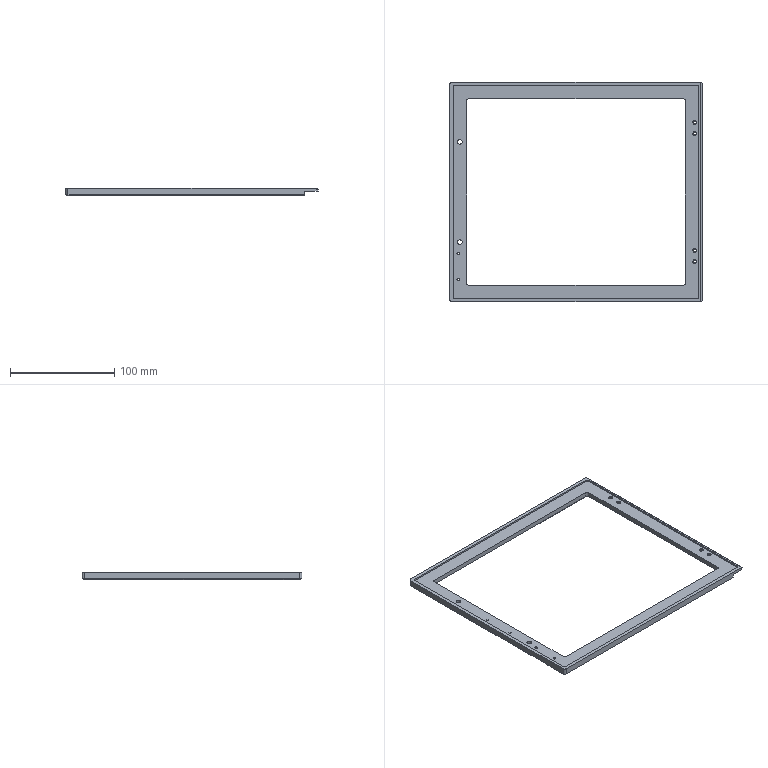NC program | NX | posted with a generic post | part box 241.5 x 210.5 x 7 mm
Lines 1 to 415 of 3179:
N10 G17 G21 G94 G90
(FLOOR_WALL , TOOL : D63)
N12 T01 M6
N14 G54
N16 G17 G0 G90 X-160.25 Y110.247 S6500 M3
N18 G43 Z30. H1
N20 Z3.
N22 G94 G1 Z0. F1500.
N24 X-157.25
N26 X157.25
N28 Y61.423
N30 X-157.25
N32 Y12.599
N34 X157.25
N36 Y-36.226
N38 X-157.25
N40 Y-85.05
N42 X157.25
N44 X160.25
N46 Z3.
N48 G0 Z30.
N50 M5
(FLOOR_WALL_1 , TOOL : D10)
N52 T10 M6
N54 G54
N56 G17 G0 G90 X4.578 Y1.6 S9500 M3
N58 G43 Z30. H10
N60 Z1.5
N62 G94 G1 X-17.1 Z0.364 F1000.
N64 Y-1.6 Z0.196
N66 X0. Z-0.7
N68 X17.1 F2500.
N70 Y1.6
N72 X-17.1
N74 Y-1.6
N76 X0.
N78 Y-6.1
N80 X21.6
N82 Y6.1
N84 X-21.6
N86 Y-6.1
N88 X0.
N90 Y-13.1
N92 X28.6
N94 Y13.1
N96 X-28.6
N98 Y-13.1
N100 X0.
N102 Y-20.1
N104 X35.6
N106 Y20.1
N108 X-35.6
N110 Y-20.1
N112 X0.
N114 Y-27.1
N116 X42.6
N118 Y27.1
N120 X-42.6
N122 Y-27.1
N124 X0.
N126 Y-34.1
N128 X49.6
N130 Y34.1
N132 X-49.6
N134 Y-34.1
N136 X0.
N138 Y-41.1
N140 X56.6
N142 Y41.1
N144 X-56.6
N146 Y-41.1
N148 X0.
N150 Y-48.1
N152 X63.6
N154 Y48.1
N156 X-63.6
N158 Y-48.1
N160 X0.
N162 Y-55.1
N164 X70.6
N166 Y55.1
N168 X-70.6
N170 Y-55.1
N172 X0.
N174 Y-62.1
N176 X77.6
N178 Y62.1
N180 X-77.6
N182 Y-62.1
N184 X0.
N186 Y-69.1
N188 X84.6
N190 Y69.1
N192 X-84.6
N194 Y-69.1
N196 X0.
N198 Y-76.1
N200 X91.6
N202 Y76.1
N204 X-91.6
N206 Y-76.1
N208 X0.
N210 Y-83.1
N212 X98.6
N214 Y83.1
N216 X-98.6
N218 Y-83.1
N220 X0.
N222 Y-90.1
N224 X105.6
N226 Y90.1
N228 X-105.6
N230 Y-90.1
N232 X0.
N234 Y-97.1
N236 X112.6
N238 Y97.1
N240 X-112.6
N242 Y-97.1
N244 X0.
N246 Z0.8
N248 G0 X4.578 Y1.6
N250 G1 X-17.1 Z-0.336 F1000.
N252 Y-1.6 Z-0.504
N254 X0. Z-1.4
N256 X17.1 F2500.
N258 Y1.6
N260 X-17.1
N262 Y-1.6
N264 X0.
N266 Y-6.1
N268 X21.6
N270 Y6.1
N272 X-21.6
N274 Y-6.1
N276 X0.
N278 Y-13.1
N280 X28.6
N282 Y13.1
N284 X-28.6
N286 Y-13.1
N288 X0.
N290 Y-20.1
N292 X35.6
N294 Y20.1
N296 X-35.6
N298 Y-20.1
N300 X0.
N302 Y-27.1
N304 X42.6
N306 Y27.1
N308 X-42.6
N310 Y-27.1
N312 X0.
N314 Y-34.1
N316 X49.6
N318 Y34.1
N320 X-49.6
N322 Y-34.1
N324 X0.
N326 Y-41.1
N328 X56.6
N330 Y41.1
N332 X-56.6
N334 Y-41.1
N336 X0.
N338 Y-48.1
N340 X63.6
N342 Y48.1
N344 X-63.6
N346 Y-48.1
N348 X0.
N350 Y-55.1
N352 X70.6
N354 Y55.1
N356 X-70.6
N358 Y-55.1
N360 X0.
N362 Y-62.1
N364 X77.6
N366 Y62.1
N368 X-77.6
N370 Y-62.1
N372 X0.
N374 Y-69.1
N376 X84.6
N378 Y69.1
N380 X-84.6
N382 Y-69.1
N384 X0.
N386 Y-76.1
N388 X91.6
N390 Y76.1
N392 X-91.6
N394 Y-76.1
N396 X0.
N398 Y-83.1
N400 X98.6
N402 Y83.1
N404 X-98.6
N406 Y-83.1
N408 X0.
N410 Y-90.1
N412 X105.6
N414 Y90.1
N416 X-105.6
N418 Y-90.1
N420 X0.
N422 Y-97.1
N424 X112.6
N426 Y97.1
N428 X-112.6
N430 Y-97.1
N432 X0.
N434 Z0.1
N436 G0 Z30.
(CAVITY_MILL , TOOL : D4)
N438 T04 M6
N440 G17 G43 G0 G90 X111.508 Y-99.4 Z30. S9500 H4 M3
N442 Z-0.071
N444 G94 G1 X111.681 Y-99.7 F1000.
N446 G3 X112.547 Y-100.2 R1.
N448 G1 X115.5 F1500.
N450 G3 X115.7 Y-100. R0.2
N452 G1 Y-97.047
N454 G3 X115.2 Y-96.181 R1.
N456 G1 X114.9 Y-96.008
N458 G0 X111.508 Y-99.4 Z-0.429
N460 G1 X111.681 Y-99.7 F1000.
N462 G3 X112.547 Y-100.2 R1.
N464 G1 X115.5 F1500.
N466 G3 X115.7 Y-100. R0.2
N468 G1 Y-97.047
N470 G3 X115.2 Y-96.181 R1.
N472 G1 X114.9 Y-96.008
N474 G0 X111.508 Y-99.4 Z-0.786
N476 G1 X111.681 Y-99.7 F1000.
N478 G3 X112.547 Y-100.2 R1.
N480 G1 X115.5 F1500.
N482 G3 X115.7 Y-100. R0.2
N484 G1 Y-97.047
N486 G3 X115.2 Y-96.181 R1.
N488 G1 X114.9 Y-96.008
N490 G0 X111.508 Y-99.4 Z-1.143
N492 G1 X111.681 Y-99.7 F1000.
N494 G3 X112.547 Y-100.2 R1.
N496 G1 X115.5 F1500.
N498 G3 X115.7 Y-100. R0.2
N500 G1 Y-97.047
N502 G3 X115.2 Y-96.181 R1.
N504 G1 X114.9 Y-96.008
N506 G0 X111.508 Y-99.4 Z-1.5
N508 G1 X111.681 Y-99.7 F1000.
N510 G3 X112.547 Y-100.2 R1.
N512 G1 X115.5 F1500.
N514 G3 X115.7 Y-100. R0.2
N516 G1 Y-97.047
N518 G3 X115.2 Y-96.181 R1.
N520 G1 X114.9 Y-96.008
N522 G0 Z30.
N524 Y96.008
N526 Z-0.071
N528 G1 X115.2 Y96.181 F1000.
N530 G3 X115.7 Y97.047 R1.
N532 G1 Y100. F1500.
N534 G3 X115.5 Y100.2 R0.2
N536 G1 X112.547
N538 G3 X111.681 Y99.7 R1.
N540 G1 X111.508 Y99.4
N542 G0 X114.9 Y96.008 Z-0.429
N544 G1 X115.2 Y96.181 F1000.
N546 G3 X115.7 Y97.047 R1.
N548 G1 Y100. F1500.
N550 G3 X115.5 Y100.2 R0.2
N552 G1 X112.547
N554 G3 X111.681 Y99.7 R1.
N556 G1 X111.508 Y99.4
N558 G0 X114.9 Y96.008 Z-0.786
N560 G1 X115.2 Y96.181 F1000.
N562 G3 X115.7 Y97.047 R1.
N564 G1 Y100. F1500.
N566 G3 X115.5 Y100.2 R0.2
N568 G1 X112.547
N570 G3 X111.681 Y99.7 R1.
N572 G1 X111.508 Y99.4
N574 G0 X114.9 Y96.008 Z-1.143
N576 G1 X115.2 Y96.181 F1000.
N578 G3 X115.7 Y97.047 R1.
N580 G1 Y100. F1500.
N582 G3 X115.5 Y100.2 R0.2
N584 G1 X112.547
N586 G3 X111.681 Y99.7 R1.
N588 G1 X111.508 Y99.4
N590 G0 X114.9 Y96.008 Z-1.5
N592 G1 X115.2 Y96.181 F1000.
N594 G3 X115.7 Y97.047 R1.
N596 G1 Y100. F1500.
N598 G3 X115.5 Y100.2 R0.2
N600 G1 X112.547
N602 G3 X111.681 Y99.7 R1.
N604 G1 X111.508 Y99.4
N606 G0 Z30.
N608 X-111.508
N610 Z-0.071
N612 G1 X-111.681 Y99.7 F1000.
N614 G3 X-112.547 Y100.2 R1.
N616 G1 X-115.5 F1500.
N618 G3 X-115.7 Y100. R0.2
N620 G1 Y97.047
N622 G3 X-115.2 Y96.181 R1.
N624 G1 X-114.9 Y96.008
N626 G0 X-111.508 Y99.4 Z-0.429
N628 G1 X-111.681 Y99.7 F1000.
N630 G3 X-112.547 Y100.2 R1.
N632 G1 X-115.5 F1500.
N634 G3 X-115.7 Y100. R0.2
N636 G1 Y97.047
N638 G3 X-115.2 Y96.181 R1.
N640 G1 X-114.9 Y96.008
N642 G0 X-111.508 Y99.4 Z-0.786
N644 G1 X-111.681 Y99.7 F1000.
N646 G3 X-112.547 Y100.2 R1.
N648 G1 X-115.5 F1500.
N650 G3 X-115.7 Y100. R0.2
N652 G1 Y97.047
N654 G3 X-115.2 Y96.181 R1.
N656 G1 X-114.9 Y96.008
N658 G0 X-111.508 Y99.4 Z-1.143
N660 G1 X-111.681 Y99.7 F1000.
N662 G3 X-112.547 Y100.2 R1.
N664 G1 X-115.5 F1500.
N666 G3 X-115.7 Y100. R0.2
N668 G1 Y97.047
N670 G3 X-115.2 Y96.181 R1.
N672 G1 X-114.9 Y96.008
N674 G0 X-111.508 Y99.4 Z-1.5
N676 G1 X-111.681 Y99.7 F1000.
N678 G3 X-112.547 Y100.2 R1.
N680 G1 X-115.5 F1500.
N682 G3 X-115.7 Y100. R0.2
N684 G1 Y97.047
N686 G3 X-115.2 Y96.181 R1.
N688 G1 X-114.9 Y96.008
N690 G0 Z30.
N692 Y-96.008
N694 Z-0.071
N696 G1 X-115.2 Y-96.181 F1000.
N698 G3 X-115.7 Y-97.047 R1.
N700 G1 Y-100. F1500.
N702 G3 X-115.5 Y-100.2 R0.2
N704 G1 X-112.547
N706 G3 X-111.681 Y-99.7 R1.
N708 G1 X-111.508 Y-99.4
N710 G0 X-114.9 Y-96.008 Z-0.429
N712 G1 X-115.2 Y-96.181 F1000.
N714 G3 X-115.7 Y-97.047 R1.
N716 G1 Y-100. F1500.
N718 G3 X-115.5 Y-100.2 R0.2
N720 G1 X-112.547
N722 G3 X-111.681 Y-99.7 R1.
N724 G1 X-111.508 Y-99.4
N726 G0 X-114.9 Y-96.008 Z-0.786
N728 G1 X-115.2 Y-96.181 F1000.
N730 G3 X-115.7 Y-97.047 R1.
N732 G1 Y-100. F1500.
N734 G3 X-115.5 Y-100.2 R0.2
N736 G1 X-112.547
N738 G3 X-111.681 Y-99.7 R1.
N740 G1 X-111.508 Y-99.4
N742 G0 X-114.9 Y-96.008 Z-1.143
N744 G1 X-115.2 Y-96.181 F1000.
N746 G3 X-115.7 Y-97.047 R1.
N748 G1 Y-100. F1500.
N750 G3 X-115.5 Y-100.2 R0.2
N752 G1 X-112.547
N754 G3 X-111.681 Y-99.7 R1.
N756 G1 X-111.508 Y-99.4
N758 G0 X-114.9 Y-96.008 Z-1.5
N760 G1 X-115.2 Y-96.181 F1000.
N762 G3 X-115.7 Y-97.047 R1.
N764 G1 Y-100. F1500.
N766 G3 X-115.5 Y-100.2 R0.2
N768 G1 X-112.547
N770 G3 X-111.681 Y-99.7 R1.
N772 G1 X-111.508 Y-99.4
N774 G0 Z30.
(ZLEVEL_PROFILE , TOOL : D4)
N776 X119.416 Y-108.004
N778 Z-5.5
N780 G1 Z-7. F1400.
N782 X119.096 Y-107.45
N784 G3 X118.75 Y-107.25 R0.4
N786 G1 X-118.75
N788 G2 X-122.75 Y-103.25 R4.
N790 G1 Y103.25
N792 G2 X-118.75 Y107.25 R4.
N794 G1 X118.75
N796 G2 X122.75 Y103.25 R4.
N798 G1 Y-103.25
N800 G2 X118.75 Y-107.25 R4.
N802 G3 X118.404 Y-107.45 R0.4
N804 G1 X118.057 Y-108.05
N806 Z-5.5
N808 G0 Z30.
N810 M5